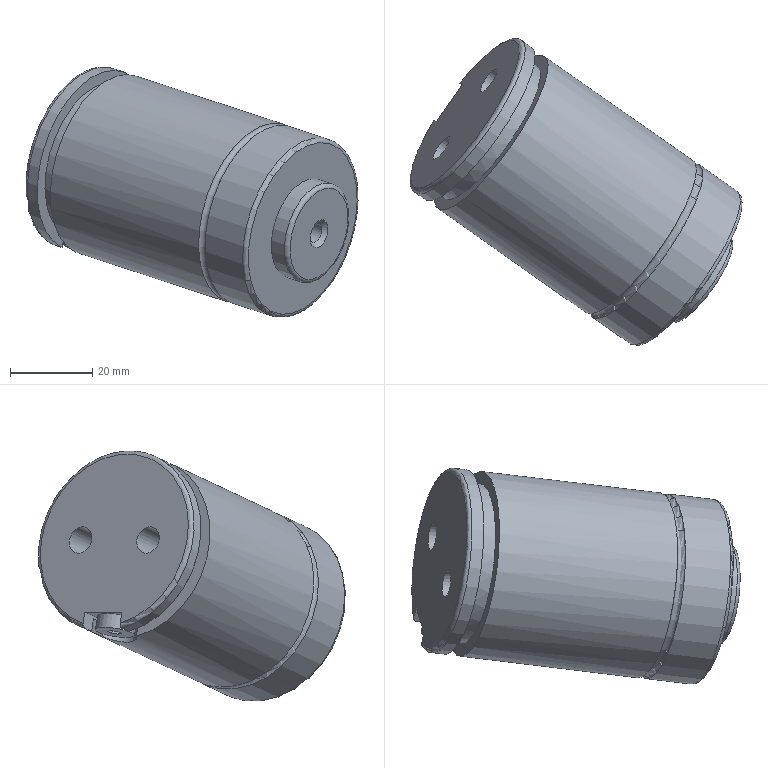Part | NX | features 1 2 | 1 solid | 34 faces | box 80.639 x 74.53 x 60.81 mm | volume 108670 mm3 | plane 16 | cylinder 10 | torus 4 | cone 4 | commonest cylinder face diameters 45.2 x3 6.6 x2 4.9 x1 9.5 x1 11 x1 25 x1
STEP:
#1=CARTESIAN_POINT('',(-319.731,837.195,-163.501));
#2=VERTEX_POINT('',#1);
#3=CARTESIAN_POINT('',(-306.768,855.708,-163.501));
#4=DIRECTION('',(0.7912,-0.554,-0.2588));
#5=DIRECTION('',(-0.5736,-0.8192,0.));
#6=AXIS2_PLACEMENT_3D('',#3,#4,#5);
#7=CIRCLE('',#6,22.6);
#8=EDGE_CURVE('',#2,#2,#7,.T.);
#9=ORIENTED_EDGE('',*,*,#8,.T.);
#10=EDGE_LOOP('',(#9));
#11=FACE_BOUND('',#10,.T.);
#12=CARTESIAN_POINT('',(-318.148,836.087,-164.018));
#13=VERTEX_POINT('',#12);
#14=CARTESIAN_POINT('',(-305.186,854.6,-164.018));
#15=DIRECTION('',(0.7912,-0.554,-0.2588));
#16=DIRECTION('',(-0.5736,-0.8192,0.));
#17=AXIS2_PLACEMENT_3D('',#14,#15,#16);
#18=CIRCLE('',#17,22.6);
#19=EDGE_CURVE('',#13,#13,#18,.T.);
#20=ORIENTED_EDGE('',*,*,#19,.F.);
#21=EDGE_LOOP('',(#20));
#22=FACE_BOUND('',#21,.T.);
#23=CARTESIAN_POINT('',(-305.977,855.154,-163.759));
#24=DIRECTION('',(0.7912,-0.554,-0.2588));
#25=DIRECTION('',(0.212,-0.1485,0.9659));
#26=AXIS2_PLACEMENT_3D('',#23,#24,#25);
#27=TOROIDAL_SURFACE('',#26,22.6,1.);
#28=ADVANCED_FACE('',(#11,#22),#27,.F.);
#29=CARTESIAN_POINT('',(-309.049,829.716,-166.995));
#30=VERTEX_POINT('',#29);
#31=CARTESIAN_POINT('',(-296.086,848.229,-166.995));
#32=DIRECTION('',(0.7912,-0.554,-0.2588));
#33=DIRECTION('',(-0.5736,-0.8192,0.));
#34=AXIS2_PLACEMENT_3D('',#31,#32,#33);
#35=CIRCLE('',#34,22.6);
#36=EDGE_CURVE('',#30,#30,#35,.T.);
#37=ORIENTED_EDGE('',*,*,#36,.T.);
#38=EDGE_LOOP('',(#37));
#39=FACE_BOUND('',#38,.T.);
#40=CARTESIAN_POINT('',(-307.684,829.981,-167.253));
#41=VERTEX_POINT('',#40);
#42=CARTESIAN_POINT('',(-295.295,847.675,-167.253));
#43=DIRECTION('',(0.7912,-0.554,-0.2588));
#44=DIRECTION('',(-0.5736,-0.8192,0.));
#45=AXIS2_PLACEMENT_3D('',#42,#43,#44);
#46=CIRCLE('',#45,21.6);
#47=EDGE_CURVE('',#41,#41,#46,.T.);
#48=ORIENTED_EDGE('',*,*,#47,.F.);
#49=EDGE_LOOP('',(#48));
#50=FACE_BOUND('',#49,.T.);
#51=CARTESIAN_POINT('',(-296.086,848.229,-166.995));
#52=DIRECTION('',(0.7912,-0.554,-0.2588));
#53=DIRECTION('',(0.212,-0.1485,0.9659));
#54=AXIS2_PLACEMENT_3D('',#51,#52,#53);
#55=TOROIDAL_SURFACE('',#54,21.6,1.);
#56=ADVANCED_FACE('',(#39,#50),#55,.T.);
#57=ORIENTED_EDGE('',*,*,#19,.T.);
#58=EDGE_LOOP('',(#57));
#59=FACE_BOUND('',#58,.T.);
#60=ORIENTED_EDGE('',*,*,#36,.F.);
#61=EDGE_LOOP('',(#60));
#62=FACE_BOUND('',#61,.T.);
#63=CARTESIAN_POINT('',(-300.636,851.414,-165.506));
#64=DIRECTION('',(-0.7912,0.554,0.2588));
#65=DIRECTION('',(-0.212,0.1485,-0.9659));
#66=AXIS2_PLACEMENT_3D('',#63,#64,#65);
#67=CYLINDRICAL_SURFACE('',#66,22.6);
#68=ADVANCED_FACE('',(#59,#62),#67,.T.);
#69=CARTESIAN_POINT('',(-299.3,835.219,-168.289));
#70=VERTEX_POINT('',#69);
#71=CARTESIAN_POINT('',(-292.13,845.458,-168.289));
#72=DIRECTION('',(0.7912,-0.554,-0.2588));
#73=DIRECTION('',(-0.5736,-0.8192,0.));
#74=AXIS2_PLACEMENT_3D('',#71,#72,#73);
#75=CIRCLE('',#74,12.5);
#76=EDGE_CURVE('',#70,#70,#75,.T.);
#77=ORIENTED_EDGE('',*,*,#76,.T.);
#78=EDGE_LOOP('',(#77));
#79=FACE_BOUND('',#78,.T.);
#80=CARTESIAN_POINT('',(-297.935,835.484,-168.548));
#81=VERTEX_POINT('',#80);
#82=CARTESIAN_POINT('',(-291.339,844.904,-168.548));
#83=DIRECTION('',(0.7912,-0.554,-0.2588));
#84=DIRECTION('',(-0.5736,-0.8192,0.));
#85=AXIS2_PLACEMENT_3D('',#82,#83,#84);
#86=CIRCLE('',#85,11.5);
#87=EDGE_CURVE('',#81,#81,#86,.T.);
#88=ORIENTED_EDGE('',*,*,#87,.F.);
#89=EDGE_LOOP('',(#88));
#90=FACE_BOUND('',#89,.T.);
#91=CARTESIAN_POINT('',(-292.13,845.458,-168.289));
#92=DIRECTION('',(0.7912,-0.554,-0.2588));
#93=DIRECTION('',(0.212,-0.1485,0.9659));
#94=AXIS2_PLACEMENT_3D('',#91,#92,#93);
#95=TOROIDAL_SURFACE('',#94,11.5,1.);
#96=ADVANCED_FACE('',(#79,#90),#95,.T.);
#97=CARTESIAN_POINT('',(-302.465,837.435,-167.253));
#98=VERTEX_POINT('',#97);
#99=CARTESIAN_POINT('',(-295.295,847.675,-167.253));
#100=DIRECTION('',(-0.7912,0.554,0.2588));
#101=DIRECTION('',(-0.5736,-0.8192,0.));
#102=AXIS2_PLACEMENT_3D('',#99,#100,#101);
#103=CIRCLE('',#102,12.5);
#104=EDGE_CURVE('',#98,#98,#103,.T.);
#105=ORIENTED_EDGE('',*,*,#104,.F.);
#106=EDGE_LOOP('',(#105));
#107=FACE_BOUND('',#106,.T.);
#108=ORIENTED_EDGE('',*,*,#76,.F.);
#109=EDGE_LOOP('',(#108));
#110=FACE_BOUND('',#109,.T.);
#111=CARTESIAN_POINT('',(-293.713,846.566,-167.771));
#112=DIRECTION('',(-0.7912,0.554,0.2588));
#113=DIRECTION('',(-0.212,0.1485,-0.9659));
#114=AXIS2_PLACEMENT_3D('',#111,#112,#113);
#115=CYLINDRICAL_SURFACE('',#114,12.5);
#116=ADVANCED_FACE('',(#107,#110),#115,.T.);
#117=CARTESIAN_POINT('',(-352.942,879.86,-149.654));
#118=VERTEX_POINT('',#117);
#119=CARTESIAN_POINT('',(-354.835,877.157,-149.654));
#120=DIRECTION('',(0.7912,-0.554,-0.2588));
#121=DIRECTION('',(0.5736,0.8192,0.));
#122=AXIS2_PLACEMENT_3D('',#119,#120,#121);
#123=CIRCLE('',#122,3.3);
#124=EDGE_CURVE('',#118,#118,#123,.T.);
#125=ORIENTED_EDGE('',*,*,#124,.F.);
#126=EDGE_LOOP('',(#125));
#127=FACE_BOUND('',#126,.T.);
#128=CARTESIAN_POINT('',(-344.081,873.655,-152.553));
#129=VERTEX_POINT('',#128);
#130=CARTESIAN_POINT('',(-345.973,870.952,-152.553));
#131=DIRECTION('',(-0.7912,0.554,0.2588));
#132=DIRECTION('',(0.5736,0.8192,0.));
#133=AXIS2_PLACEMENT_3D('',#130,#131,#132);
#134=CIRCLE('',#133,3.3);
#135=EDGE_CURVE('',#129,#129,#134,.T.);
#136=ORIENTED_EDGE('',*,*,#135,.F.);
#137=EDGE_LOOP('',(#136));
#138=FACE_BOUND('',#137,.T.);
#139=CARTESIAN_POINT('',(-350.404,874.055,-151.103));
#140=DIRECTION('',(0.7912,-0.554,-0.2588));
#141=DIRECTION('',(0.212,-0.1485,0.9659));
#142=AXIS2_PLACEMENT_3D('',#139,#140,#141);
#143=CYLINDRICAL_SURFACE('',#142,3.3);
#144=ADVANCED_FACE('',(#127,#138),#143,.F.);
#145=ORIENTED_EDGE('',*,*,#135,.T.);
#146=EDGE_LOOP('',(#145));
#147=FACE_BOUND('',#146,.T.);
#148=CARTESIAN_POINT('',(-348.11,872.448,-151.854));
#149=VERTEX_POINT('',#148);
#150=VERTEX_LOOP('',#149);
#151=FACE_BOUND('',#150,.T.);
#152=CARTESIAN_POINT('',(-347.041,871.7,-152.203));
#153=DIRECTION('',(0.7912,-0.554,-0.2588));
#154=DIRECTION('',(0.212,-0.1485,0.9659));
#155=AXIS2_PLACEMENT_3D('',#152,#153,#154);
#156=CONICAL_SURFACE('',#155,1.65,0.8851);
#157=ADVANCED_FACE('',(#147,#151),#156,.T.);
#158=CARTESIAN_POINT('',(-293.346,842.037,-168.548));
#159=VERTEX_POINT('',#158);
#160=CARTESIAN_POINT('',(-291.339,844.904,-168.548));
#161=DIRECTION('',(-0.7912,0.554,0.2588));
#162=DIRECTION('',(-0.5736,-0.8192,0.));
#163=AXIS2_PLACEMENT_3D('',#160,#161,#162);
#164=CIRCLE('',#163,3.5);
#165=EDGE_CURVE('',#159,#159,#164,.T.);
#166=ORIENTED_EDGE('',*,*,#165,.F.);
#167=EDGE_LOOP('',(#166));
#168=FACE_BOUND('',#167,.T.);
#169=CARTESIAN_POINT('',(-293.575,843.479,-168.276));
#170=VERTEX_POINT('',#169);
#171=CARTESIAN_POINT('',(-292.17,845.486,-168.276));
#172=DIRECTION('',(0.7912,-0.554,-0.2588));
#173=DIRECTION('',(-0.5736,-0.8192,0.));
#174=AXIS2_PLACEMENT_3D('',#171,#172,#173);
#175=CIRCLE('',#174,2.45);
#176=EDGE_CURVE('',#170,#170,#175,.T.);
#177=ORIENTED_EDGE('',*,*,#176,.F.);
#178=EDGE_LOOP('',(#177));
#179=FACE_BOUND('',#178,.T.);
#180=CARTESIAN_POINT('',(-291.754,845.195,-168.412));
#181=DIRECTION('',(0.7912,-0.554,-0.2588));
#182=DIRECTION('',(0.212,-0.1485,0.9659));
#183=AXIS2_PLACEMENT_3D('',#180,#181,#182);
#184=CONICAL_SURFACE('',#183,2.975,0.7854);
#185=ADVANCED_FACE('',(#168,#179),#184,.F.);
#186=ORIENTED_EDGE('',*,*,#176,.T.);
#187=EDGE_LOOP('',(#186));
#188=FACE_BOUND('',#187,.T.);
#189=CARTESIAN_POINT('',(-297.887,846.499,-166.865));
#190=VERTEX_POINT('',#189);
#191=CARTESIAN_POINT('',(-296.482,848.506,-166.865));
#192=DIRECTION('',(0.7912,-0.554,-0.2588));
#193=DIRECTION('',(-0.5736,-0.8192,0.));
#194=AXIS2_PLACEMENT_3D('',#191,#192,#193);
#195=CIRCLE('',#194,2.45);
#196=EDGE_CURVE('',#190,#190,#195,.T.);
#197=ORIENTED_EDGE('',*,*,#196,.F.);
#198=EDGE_LOOP('',(#197));
#199=FACE_BOUND('',#198,.T.);
#200=CARTESIAN_POINT('',(-294.326,846.996,-167.571));
#201=DIRECTION('',(-0.7912,0.554,0.2588));
#202=DIRECTION('',(-0.212,0.1485,-0.9659));
#203=AXIS2_PLACEMENT_3D('',#200,#201,#202);
#204=CYLINDRICAL_SURFACE('',#203,2.45);
#205=ADVANCED_FACE('',(#188,#199),#204,.F.);
#206=CARTESIAN_POINT('',(-297.273,849.06,-166.606));
#207=VERTEX_POINT('',#206);
#208=VERTEX_LOOP('',#207);
#209=FACE_BOUND('',#208,.T.);
#210=ORIENTED_EDGE('',*,*,#196,.T.);
#211=EDGE_LOOP('',(#210));
#212=FACE_BOUND('',#211,.T.);
#213=CARTESIAN_POINT('',(-296.878,848.783,-166.736));
#214=DIRECTION('',(0.7912,-0.554,-0.2588));
#215=DIRECTION('',(0.212,-0.1485,0.9659));
#216=AXIS2_PLACEMENT_3D('',#213,#214,#215);
#217=CONICAL_SURFACE('',#216,1.225,1.183);
#218=ADVANCED_FACE('',(#209,#212),#217,.F.);
#219=CARTESIAN_POINT('',(-336.638,888.831,-151.854));
#220=VERTEX_POINT('',#219);
#221=VERTEX_LOOP('',#220);
#222=FACE_BOUND('',#221,.T.);
#223=CARTESIAN_POINT('',(-336.395,884.632,-152.553));
#224=VERTEX_POINT('',#223);
#225=CARTESIAN_POINT('',(-334.502,887.335,-152.553));
#226=DIRECTION('',(0.7912,-0.554,-0.2588));
#227=DIRECTION('',(-0.5736,-0.8192,0.));
#228=AXIS2_PLACEMENT_3D('',#225,#226,#227);
#229=CIRCLE('',#228,3.3);
#230=EDGE_CURVE('',#224,#224,#229,.T.);
#231=ORIENTED_EDGE('',*,*,#230,.F.);
#232=EDGE_LOOP('',(#231));
#233=FACE_BOUND('',#232,.T.);
#234=CARTESIAN_POINT('',(-335.57,888.083,-152.203));
#235=DIRECTION('',(0.7912,-0.554,-0.2588));
#236=DIRECTION('',(0.212,-0.1485,0.9659));
#237=AXIS2_PLACEMENT_3D('',#234,#235,#236);
#238=CONICAL_SURFACE('',#237,1.65,0.8851);
#239=ADVANCED_FACE('',(#222,#233),#238,.T.);
#240=ORIENTED_EDGE('',*,*,#230,.T.);
#241=EDGE_LOOP('',(#240));
#242=FACE_BOUND('',#241,.T.);
#243=CARTESIAN_POINT('',(-345.256,890.837,-149.654));
#244=VERTEX_POINT('',#243);
#245=CARTESIAN_POINT('',(-343.364,893.54,-149.654));
#246=DIRECTION('',(0.7912,-0.554,-0.2588));
#247=DIRECTION('',(-0.5736,-0.8192,0.));
#248=AXIS2_PLACEMENT_3D('',#245,#246,#247);
#249=CIRCLE('',#248,3.3);
#250=EDGE_CURVE('',#244,#244,#249,.T.);
#251=ORIENTED_EDGE('',*,*,#250,.F.);
#252=EDGE_LOOP('',(#251));
#253=FACE_BOUND('',#252,.T.);
#254=CARTESIAN_POINT('',(-338.933,890.438,-151.103));
#255=DIRECTION('',(-0.7912,0.554,0.2588));
#256=DIRECTION('',(-0.212,0.1485,-0.9659));
#257=AXIS2_PLACEMENT_3D('',#254,#255,#256);
#258=CYLINDRICAL_SURFACE('',#257,3.3);
#259=ADVANCED_FACE('',(#242,#253),#258,.F.);
#260=CARTESIAN_POINT('',(-349.801,892.554,-171.086));
#261=VERTEX_POINT('',#260);
#262=CARTESIAN_POINT('',(-356.11,883.543,-171.086));
#263=VERTEX_POINT('',#262);
#264=CARTESIAN_POINT('',(-348.308,884.795,-149.913));
#265=DIRECTION('',(0.7912,-0.554,-0.2588));
#266=DIRECTION('',(-0.5736,-0.8192,0.));
#267=AXIS2_PLACEMENT_3D('',#264,#265,#266);
#268=CIRCLE('',#267,22.6);
#269=EDGE_CURVE('',#261,#263,#268,.T.);
#270=ORIENTED_EDGE('',*,*,#269,.T.);
#271=CARTESIAN_POINT('',(-353.737,881.881,-171.863));
#272=VERTEX_POINT('',#271);
#273=CARTESIAN_POINT('',(-354.923,882.712,-171.474));
#274=DIRECTION('',(0.7912,-0.554,-0.2588));
#275=VECTOR('',#274,1000.);
#276=LINE('',#273,#275);
#277=EDGE_CURVE('',#263,#272,#276,.T.);
#278=ORIENTED_EDGE('',*,*,#277,.T.);
#279=CARTESIAN_POINT('',(-347.427,890.892,-171.863));
#280=VERTEX_POINT('',#279);
#281=CARTESIAN_POINT('',(-345.934,883.133,-150.689));
#282=DIRECTION('',(-0.7912,0.554,0.2588));
#283=DIRECTION('',(-0.5736,-0.8192,0.));
#284=AXIS2_PLACEMENT_3D('',#281,#282,#283);
#285=CIRCLE('',#284,22.6);
#286=EDGE_CURVE('',#272,#280,#285,.T.);
#287=ORIENTED_EDGE('',*,*,#286,.T.);
#288=CARTESIAN_POINT('',(-348.614,891.723,-171.474));
#289=DIRECTION('',(-0.7912,0.554,0.2588));
#290=VECTOR('',#289,1000.);
#291=LINE('',#288,#290);
#292=EDGE_CURVE('',#280,#261,#291,.T.);
#293=ORIENTED_EDGE('',*,*,#292,.T.);
#294=EDGE_LOOP('',(#270,#278,#287,#293));
#295=FACE_BOUND('',#294,.T.);
#296=CARTESIAN_POINT('',(-327.538,870.251,-156.707));
#297=DIRECTION('',(-0.7912,0.554,0.2588));
#298=DIRECTION('',(-0.212,0.1485,-0.9659));
#299=AXIS2_PLACEMENT_3D('',#296,#297,#298);
#300=CYLINDRICAL_SURFACE('',#299,22.6);
#301=ADVANCED_FACE('',(#295),#300,.T.);
#302=CARTESIAN_POINT('',(-356.683,883.944,-169.83));
#303=VERTEX_POINT('',#302);
#304=CARTESIAN_POINT('',(-356.683,883.944,-169.83));
#305=CARTESIAN_POINT('',(-356.796,884.024,-170.349));
#306=CARTESIAN_POINT('',(-356.535,883.841,-170.947));
#307=CARTESIAN_POINT('',(-356.11,883.543,-171.086));
#308=B_SPLINE_CURVE_WITH_KNOTS('',3,(#304,#305,#306,#307),.UNSPECIFIED.,.F.,.F.,(4,4),(0.,0.001588),.UNSPECIFIED.);
#309=EDGE_CURVE('',#303,#263,#308,.T.);
#310=ORIENTED_EDGE('',*,*,#309,.T.);
#311=ORIENTED_EDGE('',*,*,#269,.F.);
#312=CARTESIAN_POINT('',(-350.373,892.955,-169.83));
#313=VERTEX_POINT('',#312);
#314=CARTESIAN_POINT('',(-349.801,892.554,-171.086));
#315=CARTESIAN_POINT('',(-350.226,892.852,-170.947));
#316=CARTESIAN_POINT('',(-350.487,893.035,-170.348));
#317=CARTESIAN_POINT('',(-350.373,892.955,-169.83));
#318=B_SPLINE_CURVE_WITH_KNOTS('',3,(#314,#315,#316,#317),.UNSPECIFIED.,.F.,.F.,(4,4),(0.,0.001588),.UNSPECIFIED.);
#319=EDGE_CURVE('',#261,#313,#318,.T.);
#320=ORIENTED_EDGE('',*,*,#319,.T.);
#321=CARTESIAN_POINT('',(-349.099,885.349,-149.654));
#322=DIRECTION('',(0.7912,-0.554,-0.2588));
#323=DIRECTION('',(-0.5736,-0.8192,0.));
#324=AXIS2_PLACEMENT_3D('',#321,#322,#323);
#325=CIRCLE('',#324,21.6);
#326=EDGE_CURVE('',#313,#303,#325,.T.);
#327=ORIENTED_EDGE('',*,*,#326,.T.);
#328=EDGE_LOOP('',(#310,#311,#320,#327));
#329=FACE_BOUND('',#328,.T.);
#330=CARTESIAN_POINT('',(-348.308,884.795,-149.913));
#331=DIRECTION('',(0.7912,-0.554,-0.2588));
#332=DIRECTION('',(0.212,-0.1485,0.9659));
#333=AXIS2_PLACEMENT_3D('',#330,#331,#332);
#334=TOROIDAL_SURFACE('',#333,21.6,1.);
#335=ADVANCED_FACE('',(#329),#334,.T.);
#336=CARTESIAN_POINT('',(-346.757,890.423,-168.81));
#337=VERTEX_POINT('',#336);
#338=CARTESIAN_POINT('',(-353.067,881.412,-168.81));
#339=VERTEX_POINT('',#338);
#340=CARTESIAN_POINT('',(-345.934,883.133,-150.689));
#341=DIRECTION('',(0.7912,-0.554,-0.2588));
#342=DIRECTION('',(-0.5736,-0.8192,0.));
#343=AXIS2_PLACEMENT_3D('',#340,#341,#342);
#344=CIRCLE('',#343,19.55);
#345=EDGE_CURVE('',#337,#339,#344,.T.);
#346=ORIENTED_EDGE('',*,*,#345,.T.);
#347=CARTESIAN_POINT('',(-351.484,880.304,-169.328));
#348=VERTEX_POINT('',#347);
#349=CARTESIAN_POINT('',(-352.275,880.858,-169.069));
#350=DIRECTION('',(0.7912,-0.554,-0.2588));
#351=VECTOR('',#350,1000.);
#352=LINE('',#349,#351);
#353=EDGE_CURVE('',#339,#348,#352,.T.);
#354=ORIENTED_EDGE('',*,*,#353,.T.);
#355=CARTESIAN_POINT('',(-349.708,879.52,-169.948));
#356=VERTEX_POINT('',#355);
#357=CARTESIAN_POINT('',(-351.484,880.304,-169.328));
#358=CARTESIAN_POINT('',(-350.936,879.921,-169.507));
#359=CARTESIAN_POINT('',(-350.345,879.661,-169.716));
#360=CARTESIAN_POINT('',(-349.708,879.52,-169.948));
#361=B_SPLINE_CURVE_WITH_KNOTS('',3,(#357,#358,#359,#360),.UNSPECIFIED.,.F.,.F.,(4,4),(0.,0.002038),.UNSPECIFIED.);
#362=EDGE_CURVE('',#348,#356,#361,.T.);
#363=ORIENTED_EDGE('',*,*,#362,.T.);
#364=CARTESIAN_POINT('',(-343.831,887.914,-169.948));
#365=VERTEX_POINT('',#364);
#366=CARTESIAN_POINT('',(-342.77,880.916,-151.724));
#367=DIRECTION('',(0.7912,-0.554,-0.2588));
#368=DIRECTION('',(-0.5736,-0.8192,0.));
#369=AXIS2_PLACEMENT_3D('',#366,#367,#368);
#370=CIRCLE('',#369,19.55);
#371=EDGE_CURVE('',#365,#356,#370,.T.);
#372=ORIENTED_EDGE('',*,*,#371,.F.);
#373=CARTESIAN_POINT('',(-345.175,889.315,-169.328));
#374=VERTEX_POINT('',#373);
#375=CARTESIAN_POINT('',(-343.831,887.914,-169.948));
#376=CARTESIAN_POINT('',(-344.18,888.465,-169.716));
#377=CARTESIAN_POINT('',(-344.627,888.931,-169.507));
#378=CARTESIAN_POINT('',(-345.175,889.315,-169.328));
#379=B_SPLINE_CURVE_WITH_KNOTS('',3,(#375,#376,#377,#378),.UNSPECIFIED.,.F.,.F.,(4,4),(0.,0.002038),.UNSPECIFIED.);
#380=EDGE_CURVE('',#365,#374,#379,.T.);
#381=ORIENTED_EDGE('',*,*,#380,.T.);
#382=CARTESIAN_POINT('',(-345.966,889.869,-169.069));
#383=DIRECTION('',(-0.7912,0.554,0.2588));
#384=VECTOR('',#383,1000.);
#385=LINE('',#382,#384);
#386=EDGE_CURVE('',#374,#337,#385,.T.);
#387=ORIENTED_EDGE('',*,*,#386,.T.);
#388=EDGE_LOOP('',(#346,#354,#363,#372,#381,#387));
#389=FACE_BOUND('',#388,.T.);
#390=CARTESIAN_POINT('',(-344.352,882.025,-151.207));
#391=DIRECTION('',(-0.7912,0.554,0.2588));
#392=DIRECTION('',(-0.212,0.1485,-0.9659));
#393=AXIS2_PLACEMENT_3D('',#390,#391,#392);
#394=CYLINDRICAL_SURFACE('',#393,19.55);
#395=ADVANCED_FACE('',(#389),#394,.T.);
#396=CARTESIAN_POINT('',(-350.375,879.987,-172.986));
#397=VERTEX_POINT('',#396);
#398=CARTESIAN_POINT('',(-344.498,888.381,-172.986));
#399=VERTEX_POINT('',#398);
#400=CARTESIAN_POINT('',(-350.375,879.987,-172.986));
#401=CARTESIAN_POINT('',(-349.346,879.759,-173.344));
#402=CARTESIAN_POINT('',(-347.204,879.977,-174.103));
#403=CARTESIAN_POINT('',(-344.536,882.157,-174.637));
#404=CARTESIAN_POINT('',(-343.405,885.385,-174.108));
#405=CARTESIAN_POINT('',(-343.931,887.492,-173.344));
#406=CARTESIAN_POINT('',(-344.498,888.381,-172.986));
#407=B_SPLINE_CURVE_WITH_KNOTS('',3,(#400,#401,#402,#403,#404,#405,#406),.UNSPECIFIED.,.F.,.F.,(4,1,1,1,4),(0.,0.003292,0.006584,0.009875,0.01317),.UNSPECIFIED.);
#408=EDGE_CURVE('',#397,#399,#407,.T.);
#409=ORIENTED_EDGE('',*,*,#408,.T.);
#410=CARTESIAN_POINT('',(-342.77,880.916,-151.724));
#411=DIRECTION('',(0.7912,-0.554,-0.2588));
#412=DIRECTION('',(-0.5736,-0.8192,0.));
#413=AXIS2_PLACEMENT_3D('',#410,#411,#412);
#414=CIRCLE('',#413,22.6);
#415=EDGE_CURVE('',#399,#397,#414,.T.);
#416=ORIENTED_EDGE('',*,*,#415,.T.);
#417=EDGE_LOOP('',(#409,#416));
#418=FACE_BOUND('',#417,.T.);
#419=ORIENTED_EDGE('',*,*,#8,.F.);
#420=EDGE_LOOP('',(#419));
#421=FACE_BOUND('',#420,.T.);
#422=CARTESIAN_POINT('',(-327.538,870.251,-156.707));
#423=DIRECTION('',(-0.7912,0.554,0.2588));
#424=DIRECTION('',(-0.212,0.1485,-0.9659));
#425=AXIS2_PLACEMENT_3D('',#422,#423,#424);
#426=CYLINDRICAL_SURFACE('',#425,22.6);
#427=ADVANCED_FACE('',(#418,#421),#426,.T.);
#428=CARTESIAN_POINT('',(-350.914,880.821,-168.69));
#429=VERTEX_POINT('',#428);
#430=CARTESIAN_POINT('',(-348.189,884.712,-168.69));
#431=DIRECTION('',(0.212,-0.1485,0.9659));
#432=DIRECTION('',(-0.5736,-0.8192,0.));
#433=AXIS2_PLACEMENT_3D('',#430,#431,#432);
#434=CIRCLE('',#433,4.75);
#435=EDGE_CURVE('',#429,#429,#434,.T.);
#436=ORIENTED_EDGE('',*,*,#435,.F.);
#437=EDGE_LOOP('',(#436));
#438=FACE_BOUND('',#437,.T.);
#439=CARTESIAN_POINT('',(-351.656,881.34,-172.071));
#440=VERTEX_POINT('',#439);
#441=CARTESIAN_POINT('',(-348.931,885.231,-172.071));
#442=DIRECTION('',(0.212,-0.1485,0.9659));
#443=DIRECTION('',(-0.5736,-0.8192,0.));
#444=AXIS2_PLACEMENT_3D('',#441,#442,#443);
#445=CIRCLE('',#444,4.75);
#446=EDGE_CURVE('',#440,#440,#445,.T.);
#447=ORIENTED_EDGE('',*,*,#446,.T.);
#448=EDGE_LOOP('',(#447));
#449=FACE_BOUND('',#448,.T.);
#450=CARTESIAN_POINT('',(-344.352,882.025,-151.207));
#451=DIRECTION('',(0.212,-0.1485,0.9659));
#452=DIRECTION('',(-0.5736,-0.8192,0.));
#453=AXIS2_PLACEMENT_3D('',#450,#451,#452);
#454=CYLINDRICAL_SURFACE('',#453,4.75);
#455=ADVANCED_FACE('',(#438,#449),#454,.T.);
#456=CARTESIAN_POINT('',(-349.417,883.74,-167.017));
#457=VERTEX_POINT('',#456);
#458=CARTESIAN_POINT('',(-349.242,885.448,-166.793));
#459=VERTEX_POINT('',#458);
#460=CARTESIAN_POINT('',(-349.417,883.74,-167.017));
#461=DIRECTION('',(0.1011,0.9864,0.1294));
#462=VECTOR('',#461,1000.);
#463=LINE('',#460,#462);
#464=EDGE_CURVE('',#457,#459,#463,.T.);
#465=ORIENTED_EDGE('',*,*,#464,.F.);
#466=CARTESIAN_POINT('',(-350.477,884.482,-171.847));
#467=VERTEX_POINT('',#466);
#468=CARTESIAN_POINT('',(-350.477,884.482,-171.847));
#469=DIRECTION('',(0.212,-0.1485,0.9659));
#470=VECTOR('',#469,1000.);
#471=LINE('',#468,#470);
#472=EDGE_CURVE('',#467,#457,#471,.T.);
#473=ORIENTED_EDGE('',*,*,#472,.F.);
#474=CARTESIAN_POINT('',(-350.302,886.191,-171.622));
#475=VERTEX_POINT('',#474);
#476=CARTESIAN_POINT('',(-350.282,886.389,-171.596));
#477=DIRECTION('',(-0.1011,-0.9864,-0.1294));
#478=VECTOR('',#477,1000.);
#479=LINE('',#476,#478);
#480=EDGE_CURVE('',#475,#467,#479,.T.);
#481=ORIENTED_EDGE('',*,*,#480,.F.);
#482=CARTESIAN_POINT('',(-350.302,886.191,-171.622));
#483=DIRECTION('',(0.212,-0.1485,0.9659));
#484=VECTOR('',#483,1000.);
#485=LINE('',#482,#484);
#486=EDGE_CURVE('',#475,#459,#485,.T.);
#487=ORIENTED_EDGE('',*,*,#486,.T.);
#488=EDGE_LOOP('',(#465,#473,#481,#487));
#489=FACE_BOUND('',#488,.T.);
#490=CARTESIAN_POINT('',(-350.477,884.482,-171.847));
#491=DIRECTION('',(-0.972,0.07023,0.2241));
#492=DIRECTION('',(-0.1011,-0.9864,-0.1294));
#493=AXIS2_PLACEMENT_3D('',#490,#491,#492);
#494=PLANE('',#493);
#495=ADVANCED_FACE('',(#489),#494,.F.);
#496=CARTESIAN_POINT('',(-347.696,886.197,-167.017));
#497=VERTEX_POINT('',#496);
#498=CARTESIAN_POINT('',(-349.242,885.448,-166.793));
#499=DIRECTION('',(0.8924,0.4324,-0.1294));
#500=VECTOR('',#499,1000.);
#501=LINE('',#498,#500);
#502=EDGE_CURVE('',#459,#497,#501,.T.);
#503=ORIENTED_EDGE('',*,*,#502,.F.);
#504=ORIENTED_EDGE('',*,*,#486,.F.);
#505=CARTESIAN_POINT('',(-348.756,886.94,-171.847));
#506=VERTEX_POINT('',#505);
#507=CARTESIAN_POINT('',(-351.254,885.729,-171.484));
#508=DIRECTION('',(-0.8924,-0.4324,0.1294));
#509=VECTOR('',#508,1000.);
#510=LINE('',#507,#509);
#511=EDGE_CURVE('',#506,#475,#510,.T.);
#512=ORIENTED_EDGE('',*,*,#511,.F.);
#513=CARTESIAN_POINT('',(-348.756,886.94,-171.847));
#514=DIRECTION('',(0.212,-0.1485,0.9659));
#515=VECTOR('',#514,1000.);
#516=LINE('',#513,#515);
#517=EDGE_CURVE('',#506,#497,#516,.T.);
#518=ORIENTED_EDGE('',*,*,#517,.T.);
#519=EDGE_LOOP('',(#503,#504,#512,#518));
#520=FACE_BOUND('',#519,.T.);
#521=CARTESIAN_POINT('',(-350.302,886.191,-171.622));
#522=DIRECTION('',(-0.3984,0.8894,0.2241));
#523=DIRECTION('',(-0.8924,-0.4324,0.1294));
#524=AXIS2_PLACEMENT_3D('',#521,#522,#523);
#525=PLANE('',#524);
#526=ADVANCED_FACE('',(#520),#525,.F.);
#527=CARTESIAN_POINT('',(-346.326,885.238,-167.465));
#528=VERTEX_POINT('',#527);
#529=CARTESIAN_POINT('',(-347.696,886.197,-167.017));
#530=DIRECTION('',(0.7912,-0.554,-0.2588));
#531=VECTOR('',#530,1000.);
#532=LINE('',#529,#531);
#533=EDGE_CURVE('',#497,#528,#532,.T.);
#534=ORIENTED_EDGE('',*,*,#533,.F.);
#535=ORIENTED_EDGE('',*,*,#517,.F.);
#536=CARTESIAN_POINT('',(-347.386,885.98,-172.295));
#537=VERTEX_POINT('',#536);
#538=CARTESIAN_POINT('',(-350.787,888.362,-171.182));
#539=DIRECTION('',(-0.7912,0.554,0.2588));
#540=VECTOR('',#539,1000.);
#541=LINE('',#538,#540);
#542=EDGE_CURVE('',#537,#506,#541,.T.);
#543=ORIENTED_EDGE('',*,*,#542,.F.);
#544=CARTESIAN_POINT('',(-347.386,885.98,-172.295));
#545=DIRECTION('',(0.212,-0.1485,0.9659));
#546=VECTOR('',#545,1000.);
#547=LINE('',#544,#546);
#548=EDGE_CURVE('',#537,#528,#547,.T.);
#549=ORIENTED_EDGE('',*,*,#548,.T.);
#550=EDGE_LOOP('',(#534,#535,#543,#549));
#551=FACE_BOUND('',#550,.T.);
#552=CARTESIAN_POINT('',(-348.756,886.94,-171.847));
#553=DIRECTION('',(0.5736,0.8192,0.));
#554=DIRECTION('',(0.212,-0.1485,0.9659));
#555=AXIS2_PLACEMENT_3D('',#552,#553,#554);
#556=PLANE('',#555);
#557=ADVANCED_FACE('',(#551),#556,.F.);
#558=CARTESIAN_POINT('',(-346.501,883.529,-167.689));
#559=VERTEX_POINT('',#558);
#560=CARTESIAN_POINT('',(-346.326,885.238,-167.465));
#561=DIRECTION('',(-0.1011,-0.9864,-0.1294));
#562=VECTOR('',#561,1000.);
#563=LINE('',#560,#562);
#564=EDGE_CURVE('',#528,#559,#563,.T.);
#565=ORIENTED_EDGE('',*,*,#564,.F.);
#566=ORIENTED_EDGE('',*,*,#548,.F.);
#567=CARTESIAN_POINT('',(-347.561,884.271,-172.519));
#568=VERTEX_POINT('',#567);
#569=CARTESIAN_POINT('',(-347.278,887.033,-172.157));
#570=DIRECTION('',(0.1011,0.9864,0.1294));
#571=VECTOR('',#570,1000.);
#572=LINE('',#569,#571);
#573=EDGE_CURVE('',#568,#537,#572,.T.);
#574=ORIENTED_EDGE('',*,*,#573,.F.);
#575=CARTESIAN_POINT('',(-347.561,884.271,-172.519));
#576=DIRECTION('',(0.212,-0.1485,0.9659));
#577=VECTOR('',#576,1000.);
#578=LINE('',#575,#577);
#579=EDGE_CURVE('',#568,#559,#578,.T.);
#580=ORIENTED_EDGE('',*,*,#579,.T.);
#581=EDGE_LOOP('',(#565,#566,#574,#580));
#582=FACE_BOUND('',#581,.T.);
#583=CARTESIAN_POINT('',(-347.386,885.98,-172.295));
#584=DIRECTION('',(0.972,-0.07023,-0.2241));
#585=DIRECTION('',(0.1011,0.9864,0.1294));
#586=AXIS2_PLACEMENT_3D('',#583,#584,#585);
#587=PLANE('',#586);
#588=ADVANCED_FACE('',(#582),#587,.F.);
#589=CARTESIAN_POINT('',(-348.047,882.78,-167.465));
#590=VERTEX_POINT('',#589);
#591=CARTESIAN_POINT('',(-346.501,883.529,-167.689));
#592=DIRECTION('',(-0.8924,-0.4324,0.1294));
#593=VECTOR('',#592,1000.);
#594=LINE('',#591,#593);
#595=EDGE_CURVE('',#559,#590,#594,.T.);
#596=ORIENTED_EDGE('',*,*,#595,.F.);
#597=ORIENTED_EDGE('',*,*,#579,.F.);
#598=CARTESIAN_POINT('',(-349.107,883.523,-172.295));
#599=VERTEX_POINT('',#598);
#600=CARTESIAN_POINT('',(-349.286,883.436,-172.269));
#601=DIRECTION('',(0.8924,0.4324,-0.1294));
#602=VECTOR('',#601,1000.);
#603=LINE('',#600,#602);
#604=EDGE_CURVE('',#599,#568,#603,.T.);
#605=ORIENTED_EDGE('',*,*,#604,.F.);
#606=CARTESIAN_POINT('',(-349.107,883.523,-172.295));
#607=DIRECTION('',(0.212,-0.1485,0.9659));
#608=VECTOR('',#607,1000.);
#609=LINE('',#606,#608);
#610=EDGE_CURVE('',#599,#590,#609,.T.);
#611=ORIENTED_EDGE('',*,*,#610,.T.);
#612=EDGE_LOOP('',(#596,#597,#605,#611));
#613=FACE_BOUND('',#612,.T.);
#614=CARTESIAN_POINT('',(-347.561,884.271,-172.519));
#615=DIRECTION('',(0.3984,-0.8894,-0.2241));
#616=DIRECTION('',(0.8924,0.4324,-0.1294));
#617=AXIS2_PLACEMENT_3D('',#614,#615,#616);
#618=PLANE('',#617);
#619=ADVANCED_FACE('',(#613),#618,.F.);
#620=CARTESIAN_POINT('',(-348.047,882.78,-167.465));
#621=DIRECTION('',(-0.7912,0.554,0.2588));
#622=VECTOR('',#621,1000.);
#623=LINE('',#620,#622);
#624=EDGE_CURVE('',#590,#457,#623,.T.);
#625=ORIENTED_EDGE('',*,*,#624,.F.);
#626=ORIENTED_EDGE('',*,*,#610,.F.);
#627=CARTESIAN_POINT('',(-351.823,885.425,-171.406));
#628=DIRECTION('',(0.7912,-0.554,-0.2588));
#629=VECTOR('',#628,1000.);
#630=LINE('',#627,#629);
#631=EDGE_CURVE('',#467,#599,#630,.T.);
#632=ORIENTED_EDGE('',*,*,#631,.F.);
#633=ORIENTED_EDGE('',*,*,#472,.T.);
#634=EDGE_LOOP('',(#625,#626,#632,#633));
#635=FACE_BOUND('',#634,.T.);
#636=CARTESIAN_POINT('',(-349.107,883.523,-172.295));
#637=DIRECTION('',(-0.5736,-0.8192,0.));
#638=DIRECTION('',(-0.212,0.1485,-0.9659));
#639=AXIS2_PLACEMENT_3D('',#636,#637,#638);
#640=PLANE('',#639);
#641=ADVANCED_FACE('',(#635),#640,.F.);
#642=ORIENTED_EDGE('',*,*,#464,.T.);
#643=ORIENTED_EDGE('',*,*,#502,.T.);
#644=ORIENTED_EDGE('',*,*,#533,.T.);
#645=ORIENTED_EDGE('',*,*,#564,.T.);
#646=ORIENTED_EDGE('',*,*,#595,.T.);
#647=ORIENTED_EDGE('',*,*,#624,.T.);
#648=EDGE_LOOP('',(#642,#643,#644,#645,#646,#647));
#649=FACE_BOUND('',#648,.T.);
#650=CARTESIAN_POINT('',(-347.871,884.489,-167.241));
#651=DIRECTION('',(-0.212,0.1485,-0.9659));
#652=DIRECTION('',(0.5736,0.8192,0.));
#653=AXIS2_PLACEMENT_3D('',#650,#651,#652);
#654=PLANE('',#653);
#655=ADVANCED_FACE('',(#649),#654,.T.);
#656=ORIENTED_EDGE('',*,*,#480,.T.);
#657=ORIENTED_EDGE('',*,*,#631,.T.);
#658=ORIENTED_EDGE('',*,*,#604,.T.);
#659=ORIENTED_EDGE('',*,*,#573,.T.);
#660=ORIENTED_EDGE('',*,*,#542,.T.);
#661=ORIENTED_EDGE('',*,*,#511,.T.);
#662=EDGE_LOOP('',(#656,#657,#658,#659,#660,#661));
#663=FACE_BOUND('',#662,.T.);
#664=ORIENTED_EDGE('',*,*,#446,.F.);
#665=EDGE_LOOP('',(#664));
#666=FACE_BOUND('',#665,.T.);
#667=CARTESIAN_POINT('',(-353.679,888.555,-170.518));
#668=DIRECTION('',(0.212,-0.1485,0.9659));
#669=DIRECTION('',(-0.5736,-0.8192,0.));
#670=AXIS2_PLACEMENT_3D('',#667,#668,#669);
#671=PLANE('',#670);
#672=ADVANCED_FACE('',(#663,#666),#671,.F.);
#673=ORIENTED_EDGE('',*,*,#380,.F.);
#674=CARTESIAN_POINT('',(-344.145,888.134,-171.381));
#675=DIRECTION('',(0.212,-0.1485,0.9659));
#676=VECTOR('',#675,1000.);
#677=LINE('',#674,#676);
#678=EDGE_CURVE('',#399,#365,#677,.T.);
#679=ORIENTED_EDGE('',*,*,#678,.F.);
#680=ORIENTED_EDGE('',*,*,#408,.F.);
#681=CARTESIAN_POINT('',(-350.023,879.741,-171.381));
#682=DIRECTION('',(-0.212,0.1485,-0.9659));
#683=VECTOR('',#682,1000.);
#684=LINE('',#681,#683);
#685=EDGE_CURVE('',#356,#397,#684,.T.);
#686=ORIENTED_EDGE('',*,*,#685,.F.);
#687=ORIENTED_EDGE('',*,*,#362,.F.);
#688=CARTESIAN_POINT('',(-351.344,880.206,-168.69));
#689=VERTEX_POINT('',#688);
#690=CARTESIAN_POINT('',(-352.298,880.874,-173.037));
#691=DIRECTION('',(0.212,-0.1485,0.9659));
#692=VECTOR('',#691,1000.);
#693=LINE('',#690,#692);
#694=EDGE_CURVE('',#348,#689,#693,.T.);
#695=ORIENTED_EDGE('',*,*,#694,.T.);
#696=CARTESIAN_POINT('',(-345.035,889.217,-168.69));
#697=VERTEX_POINT('',#696);
#698=CARTESIAN_POINT('',(-348.189,884.712,-168.69));
#699=DIRECTION('',(-0.212,0.1485,-0.9659));
#700=DIRECTION('',(-0.5736,-0.8192,0.));
#701=AXIS2_PLACEMENT_3D('',#698,#699,#700);
#702=CIRCLE('',#701,5.5);
#703=EDGE_CURVE('',#697,#689,#702,.T.);
#704=ORIENTED_EDGE('',*,*,#703,.F.);
#705=CARTESIAN_POINT('',(-345.989,889.885,-173.037));
#706=DIRECTION('',(0.212,-0.1485,0.9659));
#707=VECTOR('',#706,1000.);
#708=LINE('',#705,#707);
#709=EDGE_CURVE('',#374,#697,#708,.T.);
#710=ORIENTED_EDGE('',*,*,#709,.F.);
#711=EDGE_LOOP('',(#673,#679,#680,#686,#687,#695,#704,#710));
#712=FACE_BOUND('',#711,.T.);
#713=CARTESIAN_POINT('',(-349.143,885.38,-173.037));
#714=DIRECTION('',(-0.212,0.1485,-0.9659));
#715=DIRECTION('',(0.5736,0.8192,0.));
#716=AXIS2_PLACEMENT_3D('',#713,#714,#715);
#717=CYLINDRICAL_SURFACE('',#716,5.5);
#718=ADVANCED_FACE('',(#712),#717,.F.);
#719=ORIENTED_EDGE('',*,*,#386,.F.);
#720=ORIENTED_EDGE('',*,*,#709,.T.);
#721=CARTESIAN_POINT('',(-349.782,892.541,-167.137));
#722=VERTEX_POINT('',#721);
#723=CARTESIAN_POINT('',(-345.035,889.217,-168.69));
#724=DIRECTION('',(0.7912,-0.554,-0.2588));
#725=VECTOR('',#724,1000.);
#726=LINE('',#723,#725);
#727=EDGE_CURVE('',#722,#697,#726,.T.);
#728=ORIENTED_EDGE('',*,*,#727,.F.);
#729=CARTESIAN_POINT('',(-348.34,891.532,-160.569));
#730=DIRECTION('',(0.212,-0.1485,0.9659));
#731=VECTOR('',#730,1000.);
#732=LINE('',#729,#731);
#733=EDGE_CURVE('',#313,#722,#732,.T.);
#734=ORIENTED_EDGE('',*,*,#733,.F.);
#735=ORIENTED_EDGE('',*,*,#319,.F.);
#736=ORIENTED_EDGE('',*,*,#292,.F.);
#737=CARTESIAN_POINT('',(-345.176,889.315,-161.604));
#738=DIRECTION('',(-0.212,0.1485,-0.9659));
#739=VECTOR('',#738,1000.);
#740=LINE('',#737,#739);
#741=EDGE_CURVE('',#337,#280,#740,.T.);
#742=ORIENTED_EDGE('',*,*,#741,.F.);
#743=EDGE_LOOP('',(#719,#720,#728,#734,#735,#736,#742));
#744=FACE_BOUND('',#743,.T.);
#745=CARTESIAN_POINT('',(-350.736,893.209,-171.484));
#746=DIRECTION('',(0.5736,0.8192,0.));
#747=DIRECTION('',(0.212,-0.1485,0.9659));
#748=AXIS2_PLACEMENT_3D('',#745,#746,#747);
#749=PLANE('',#748);
#750=ADVANCED_FACE('',(#744),#749,.F.);
#751=ORIENTED_EDGE('',*,*,#353,.F.);
#752=CARTESIAN_POINT('',(-351.485,880.305,-161.604));
#753=DIRECTION('',(0.212,-0.1485,0.9659));
#754=VECTOR('',#753,1000.);
#755=LINE('',#752,#754);
#756=EDGE_CURVE('',#272,#339,#755,.T.);
#757=ORIENTED_EDGE('',*,*,#756,.F.);
#758=ORIENTED_EDGE('',*,*,#277,.F.);
#759=ORIENTED_EDGE('',*,*,#309,.F.);
#760=CARTESIAN_POINT('',(-356.092,883.53,-167.137));
#761=VERTEX_POINT('',#760);
#762=CARTESIAN_POINT('',(-354.65,882.521,-160.569));
#763=DIRECTION('',(-0.212,0.1485,-0.9659));
#764=VECTOR('',#763,1000.);
#765=LINE('',#762,#764);
#766=EDGE_CURVE('',#761,#303,#765,.T.);
#767=ORIENTED_EDGE('',*,*,#766,.F.);
#768=CARTESIAN_POINT('',(-356.092,883.53,-167.137));
#769=DIRECTION('',(-0.7912,0.554,0.2588));
#770=VECTOR('',#769,1000.);
#771=LINE('',#768,#770);
#772=EDGE_CURVE('',#689,#761,#771,.T.);
#773=ORIENTED_EDGE('',*,*,#772,.F.);
#774=ORIENTED_EDGE('',*,*,#694,.F.);
#775=EDGE_LOOP('',(#751,#757,#758,#759,#767,#773,#774));
#776=FACE_BOUND('',#775,.T.);
#777=CARTESIAN_POINT('',(-352.298,880.874,-173.037));
#778=DIRECTION('',(-0.5736,-0.8192,0.));
#779=DIRECTION('',(-0.212,0.1485,-0.9659));
#780=AXIS2_PLACEMENT_3D('',#777,#778,#779);
#781=PLANE('',#780);
#782=ADVANCED_FACE('',(#776),#781,.F.);
#783=ORIENTED_EDGE('',*,*,#435,.T.);
#784=EDGE_LOOP('',(#783));
#785=FACE_BOUND('',#784,.T.);
#786=ORIENTED_EDGE('',*,*,#727,.T.);
#787=ORIENTED_EDGE('',*,*,#703,.T.);
#788=ORIENTED_EDGE('',*,*,#772,.T.);
#789=CARTESIAN_POINT('',(-356.034,883.612,-167.137));
#790=DIRECTION('',(-0.5736,-0.8192,0.));
#791=VECTOR('',#790,1000.);
#792=LINE('',#789,#791);
#793=EDGE_CURVE('',#722,#761,#792,.T.);
#794=ORIENTED_EDGE('',*,*,#793,.F.);
#795=EDGE_LOOP('',(#786,#787,#788,#794));
#796=FACE_BOUND('',#795,.T.);
#797=CARTESIAN_POINT('',(-352.937,888.036,-167.137));
#798=DIRECTION('',(0.212,-0.1485,0.9659));
#799=DIRECTION('',(-0.5736,-0.8192,0.));
#800=AXIS2_PLACEMENT_3D('',#797,#798,#799);
#801=PLANE('',#800);
#802=ADVANCED_FACE('',(#785,#796),#801,.F.);
#803=ORIENTED_EDGE('',*,*,#678,.T.);
#804=ORIENTED_EDGE('',*,*,#371,.T.);
#805=ORIENTED_EDGE('',*,*,#685,.T.);
#806=ORIENTED_EDGE('',*,*,#415,.F.);
#807=EDGE_LOOP('',(#803,#804,#805,#806));
#808=FACE_BOUND('',#807,.T.);
#809=CARTESIAN_POINT('',(-354.915,863.571,-151.724));
#810=DIRECTION('',(0.7912,-0.554,-0.2588));
#811=DIRECTION('',(0.212,-0.1485,0.9659));
#812=AXIS2_PLACEMENT_3D('',#809,#810,#811);
#813=PLANE('',#812);
#814=ADVANCED_FACE('',(#808),#813,.F.);
#815=ORIENTED_EDGE('',*,*,#741,.T.);
#816=ORIENTED_EDGE('',*,*,#286,.F.);
#817=ORIENTED_EDGE('',*,*,#756,.T.);
#818=ORIENTED_EDGE('',*,*,#345,.F.);
#819=EDGE_LOOP('',(#815,#816,#817,#818));
#820=FACE_BOUND('',#819,.T.);
#821=CARTESIAN_POINT('',(-358.08,865.787,-150.689));
#822=DIRECTION('',(-0.7912,0.554,0.2588));
#823=DIRECTION('',(-0.212,0.1485,-0.9659));
#824=AXIS2_PLACEMENT_3D('',#821,#822,#823);
#825=PLANE('',#824);
#826=ADVANCED_FACE('',(#820),#825,.F.);
#827=ORIENTED_EDGE('',*,*,#733,.T.);
#828=ORIENTED_EDGE('',*,*,#793,.T.);
#829=ORIENTED_EDGE('',*,*,#766,.T.);
#830=ORIENTED_EDGE('',*,*,#326,.F.);
#831=EDGE_LOOP('',(#827,#828,#829,#830));
#832=FACE_BOUND('',#831,.T.);
#833=ORIENTED_EDGE('',*,*,#124,.T.);
#834=EDGE_LOOP('',(#833));
#835=FACE_BOUND('',#834,.T.);
#836=ORIENTED_EDGE('',*,*,#250,.T.);
#837=EDGE_LOOP('',(#836));
#838=FACE_BOUND('',#837,.T.);
#839=CARTESIAN_POINT('',(-355.294,876.502,-149.654));
#840=DIRECTION('',(-0.7912,0.554,0.2588));
#841=DIRECTION('',(-0.5736,-0.8192,0.));
#842=AXIS2_PLACEMENT_3D('',#839,#840,#841);
#843=PLANE('',#842);
#844=ADVANCED_FACE('',(#832,#835,#838),#843,.T.);
#845=ORIENTED_EDGE('',*,*,#165,.T.);
#846=EDGE_LOOP('',(#845));
#847=FACE_BOUND('',#846,.T.);
#848=ORIENTED_EDGE('',*,*,#87,.T.);
#849=EDGE_LOOP('',(#848));
#850=FACE_BOUND('',#849,.T.);
#851=CARTESIAN_POINT('',(-294.637,840.194,-168.548));
#852=DIRECTION('',(0.7912,-0.554,-0.2588));
#853=DIRECTION('',(0.212,-0.1485,0.9659));
#854=AXIS2_PLACEMENT_3D('',#851,#852,#853);
#855=PLANE('',#854);
#856=ADVANCED_FACE('',(#847,#850),#855,.T.);
#857=ORIENTED_EDGE('',*,*,#104,.T.);
#858=EDGE_LOOP('',(#857));
#859=FACE_BOUND('',#858,.T.);
#860=ORIENTED_EDGE('',*,*,#47,.T.);
#861=EDGE_LOOP('',(#860));
#862=FACE_BOUND('',#861,.T.);
#863=CARTESIAN_POINT('',(-301.49,838.828,-167.253));
#864=DIRECTION('',(0.7912,-0.554,-0.2588));
#865=DIRECTION('',(0.212,-0.1485,0.9659));
#866=AXIS2_PLACEMENT_3D('',#863,#864,#865);
#867=PLANE('',#866);
#868=ADVANCED_FACE('',(#859,#862),#867,.T.);
#869=CLOSED_SHELL('',(#28,#56,#68,#96,#116,#144,#157,#185,#205,#218,#239,#259,#301,#335,#395,#427,#455,#495,#526,#557,#588,#619,#641,#655,#672,#718,#750,#782,#802,#814,#826,#844,#856,#868));
#870=MANIFOLD_SOLID_BREP('',#869);
#871=(LENGTH_UNIT()NAMED_UNIT(*)SI_UNIT(.MILLI.,.METRE.));
#872=UNCERTAINTY_MEASURE_WITH_UNIT(LENGTH_MEASURE(0.0508),#871,'','');
#873=(NAMED_UNIT(*)PLANE_ANGLE_UNIT()SI_UNIT($,.RADIAN.));
#874=(NAMED_UNIT(*)SI_UNIT($,.STERADIAN.)SOLID_ANGLE_UNIT());
#875=(GEOMETRIC_REPRESENTATION_CONTEXT(3)GLOBAL_UNCERTAINTY_ASSIGNED_CONTEXT((#872))GLOBAL_UNIT_ASSIGNED_CONTEXT((#871,#873,#874))REPRESENTATION_CONTEXT('',''));
#876=ADVANCED_BREP_SHAPE_REPRESENTATION('',(#870),#875);